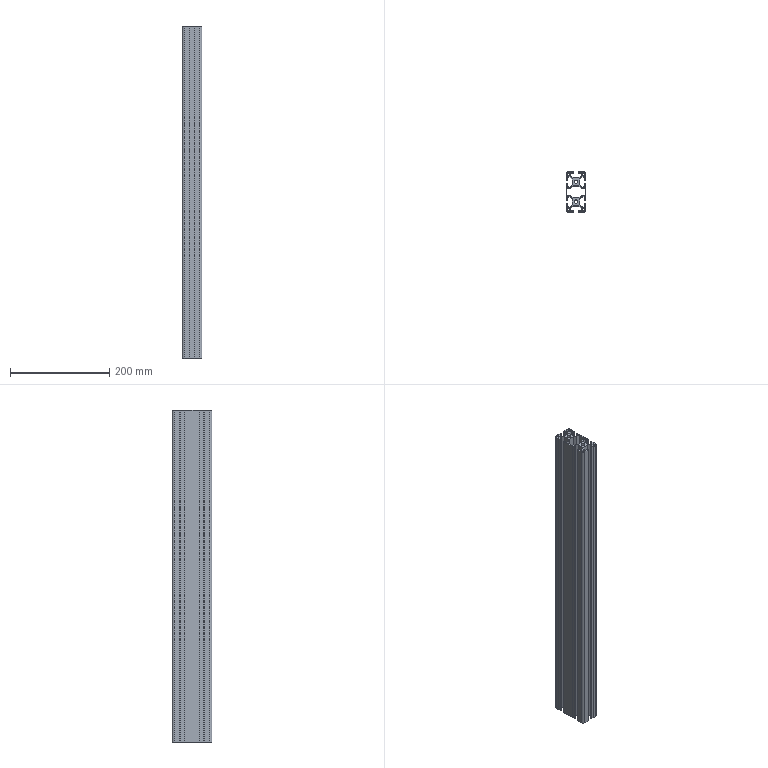Part | SolidWorks | features BaseBody 1 | 1 solid | 155 faces | box 40.002 x 80 x 670 mm | volume 659543 mm3 | plane 142 | cylinder 13 | commonest cylinder face diameters 9 x5 5 x4 6.8 x4